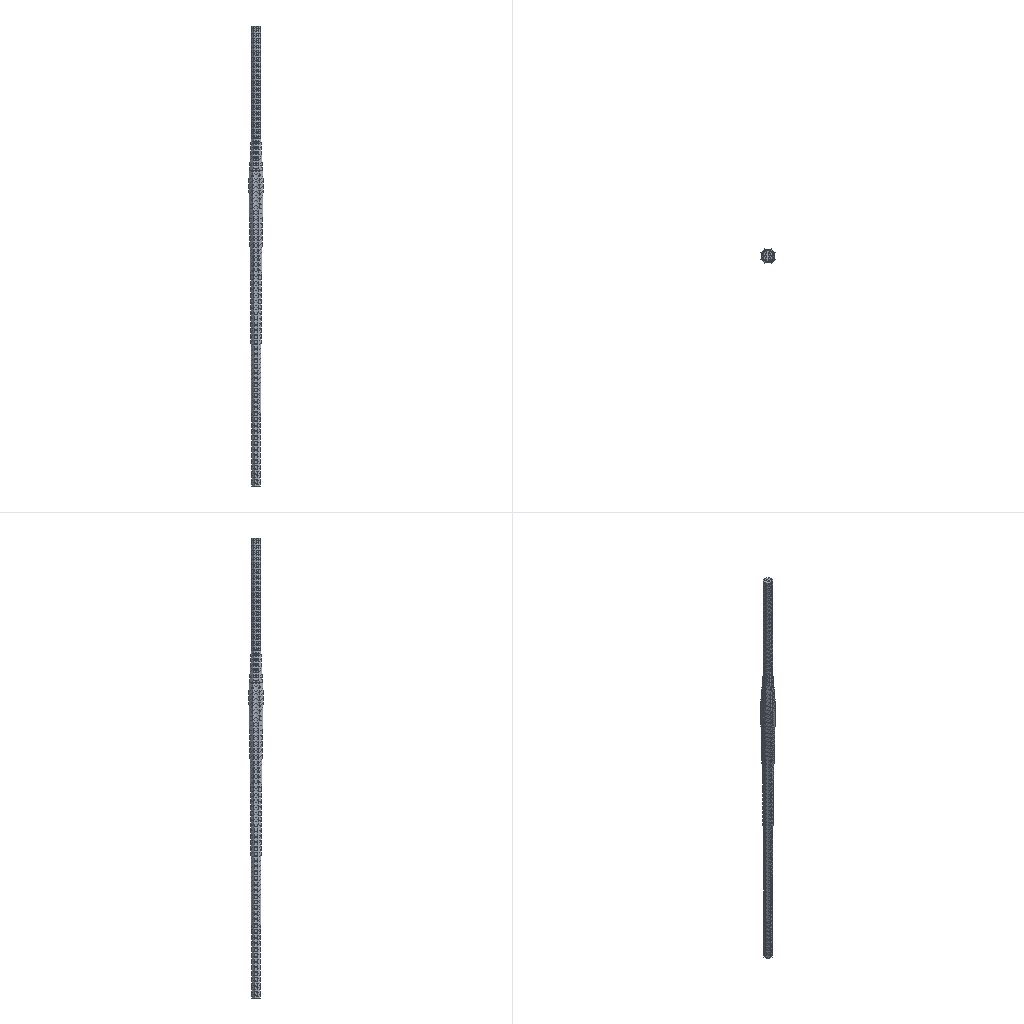Simulation study | abaqus
Set-up summary:
category,name,step,type,value,unit,region
solver,abaqus
solver,version,,,Abaqus/Explicit 2020
units,not stated in the deck,,not stated
analysis,deck,,transient,transient
load_step,Step-1,Step-1,transient,nlgeom=True
contact,interactions,,,general=0 pairs=1 ties=0
load_step,requested,,,1
mesh,nodes,,,15796
mesh,elements,,,8700
element_type,R3D3,,rigid,14
element_type,R3D4,,rigid,1363
element_type,C3D10M,,solid,7323
load,load commands in deck,,count,1
bc,support commands in deck,,count,6
material,MATERIAL-1,,in results
check,setup vs results,,match,"per instance, exact: element labels, types and connectivity; labels of the nodes the elements use; coordinates of those nodes at SINGLE_PRECISION in 1 of 2 instance(s)"
Abaqus input file, long lists of numbers shortened:
*Heading
** Job name: Job-3 Model name: Model-1-Copy2
** Generated by: Abaqus/CAE 2020
*Preprint, echo=NO, model=NO, history=NO, contact=NO
**
** PARTS
**
*Part, name="Men Surface v1"
*Node
      1,         -60.,  -26.267,   112.347
      2,          60.,  -26.267,   112.347
** (1370 more lines like these left out)
*Element, type=R3D4
 1,   1,  13, 183,  30
 2,  13,  14, 184, 183
** (1361 more lines like these left out)
*Element, type=R3D3
604,  837,  861,  875
605, 1000,  919,  815
** (12 more lines like these left out)
*Node
   1373,           0.,  -142.754,  -4.552
*Nset, nset="Men Surface v1-RefPt_", internal
1373,
*Elset, elset="Men Surface v1", generate
    1,  1377,     1
*End Part
**
*Part, name="Shinai Koto v4"
*Node
      1,         -13.,           0.,           0.
      2,   5.495,  -11.781,         300.
** (14421 more lines like these left out)
*Element, type=C3D10M
   1,  2089,  1420,  2090,  1417,  2506,  2505,  2504,  2508,  2507,  2509
   2,  2089,  2090,  2091,  2092,  2504,  2511,  2510,  2513,  2512,  2514
** (7321 more lines like these left out)
*Nset, nset=Set-4, generate
     1,  14423,      1
*Elset, elset=Set-4, generate
    1,  7323,     1
*Orientation, name=Ori-1
1., 0., 0., 0., 1., 0.
1, 0.
** Section: Section-1
*Solid Section, elset=Set-4, orientation=Ori-1, material=Material-1
,
*End Part
**
**
** ASSEMBLY
**
*Assembly, name=Assembly
**
*Instance, name="Men Surface v1-1", part="Men Surface v1"
1.74822750328583e-14, -167.849, 62.883
1.74822750328583e-14, -167.849, 62.883, 1.75414209299603e-14, -166.883, 63.142,         180.
*End Instance
**
*Instance, name="Shinai Koto v4-1", part="Shinai Koto v4"
          0.,           0.,         950.
          0.,           0.,         950.,           1.,           0.,         950.,         180.
*End Instance
**
*Nset, nset=Set-4, instance="Men Surface v1-1"
 1373,
*Nset, nset=Set-5, instance="Shinai Koto v4-1"
     4,     5,     8,     9,    12,    13,    20,    21,    26,    27,    28,    29,    30,    31,    32,    33
    34,    35,    36,    37,    38,    39,    40,    41,    42,    43,    44,    45,    46,    47,    48,    49
** (397 more lines like these left out)
*Elset, elset=Set-5, instance="Shinai Koto v4-1"
   74,  145,  149,  150,  152,  154,  155,  156,  170,  172,  175,  176,  178,  183,  184,  186
  187,  188,  190,  191,  192,  195,  197,  206,  207,  210,  211,  212,  213,  215,  216,  217
** (194 more lines like these left out)
*Nset, nset=Set-6, instance="Shinai Koto v4-1"
     1,     2,     3,     6,     7,    10,    11,    18,    19,    22,    23,    24,    25,   106,   107,   108
   109,   110,   111,   112,   113,   114,   115,   116,   181,   182,   183,   184,   185,   186,   187,   188
** (71 more lines like these left out)
*Elset, elset=Set-6, instance="Shinai Koto v4-1"
   58,   80,   92,  102,  121,  331,  422,  555,  606,  614,  701,  723,  813, 1010, 1070, 1108
 1201, 1368, 1370, 1381, 1385, 1535, 1542, 1651, 1807, 1834, 2154, 2190, 2191, 2199, 2291, 2295
** (34 more lines like these left out)
*Nset, nset=Set-7, instance="Shinai Koto v4-1"
     1,   106,   107,   108,   109,   110,   111,   112,   113,   114,   115,   116,  1771,  1772,  1773,  1774
  1775,  1776,  1777,  8271,  8284,  8288,  8291,  8772,  8775,  8783,  8810,  8816,  9594,  9596,  9598,  9639
** (2 more lines like these left out)
*Elset, elset=Set-7, instance="Shinai Koto v4-1"
 2154, 2461, 2526, 2534, 2898, 2961, 2986, 2988, 2992, 2996, 2997, 3004, 3005, 3010, 3012, 3016
 3025, 3027, 3034, 3042, 3051, 3633, 3635, 3669
*Elset, elset=_m_Surf-1_SPOS, internal, instance="Men Surface v1-1", generate
    1,  1377,     1
*Surface, type=ELEMENT, name=m_Surf-1
_m_Surf-1_SPOS, SPOS
*Elset, elset=_s_Surf-3_S3, internal, instance="Shinai Koto v4-1"
   47,   58,   74,  102,  121,  145,  149,  150,  152,  154,  155,  156,  160,  161,  165,  168
  170,  172,  175,  176,  178,  183,  184,  186,  187,  188,  190,  191,  192,  195,  206,  207
** (245 more lines like these left out)
*Elset, elset=_s_Surf-3_S2, internal, instance="Shinai Koto v4-1"
  289,  751,  759,  885,  935, 1538, 1974, 2199, 2295, 2330, 2377, 2487, 2507, 2731, 2734, 2891
 3137, 3167, 3267, 3284, 3349, 3364, 3373, 3388, 3450, 3542, 3700, 3747, 3778, 3850, 3943, 3957
** (3 more lines like these left out)
*Elset, elset=_s_Surf-3_S1, internal, instance="Shinai Koto v4-1"
  285,  286,  297,  817, 1201, 1428, 2132, 2155, 2276, 2371, 2563, 2592, 2599, 2726, 2933, 3082
 3132, 3149, 3192, 3257, 3262, 3287, 3358, 3373, 3399, 3420, 3453, 3454, 3455, 3457, 3594, 3599
** (4 more lines like these left out)
*Elset, elset=_s_Surf-3_S4, internal, instance="Shinai Koto v4-1"
   80,   92,  197,  295,  556,  562,  589,  606,  614,  701,  715, 1010, 1070, 1535, 1613, 1651
 1807, 1834, 2133, 2207, 2291, 2346, 2358, 2360, 2367, 2373, 2401, 2420, 2502, 2511, 2624, 2821
** (4 more lines like these left out)
*Surface, type=ELEMENT, name=s_Surf-3
_s_Surf-3_S3, S3
_s_Surf-3_S2, S2
_s_Surf-3_S4, S4
_s_Surf-3_S1, S1
*Rigid Body, ref node="Men Surface v1-1"."Men Surface v1-RefPt_", elset="Men Surface v1-1"."Men Surface v1"
*End Assembly
**
** MATERIALS
**
*Material, name=Material-1
*Density
 1e-09,
*Elastic, type=ENGINEERING CONSTANTS
20000., 2485.,20000.,  0.35,  0.35,   0.3, 7588., 1000.
 1000.,
**
** INTERACTION PROPERTIES
**
*Surface Interaction, name=IntProp-1
*Friction
 0.1,
*Surface Behavior, pressure-overclosure=HARD
**
** PREDEFINED FIELDS
**
** Name: Predefined Field-1   Type: Velocity
*Initial Conditions, type=ROTATING VELOCITY
Set-5, -100.,  ,  ,  ,
0., 0., 950., 1., 0., 950.,
** ----------------------------------------------------------------
**
** STEP: Step-1
**
*Step, name=Step-1, nlgeom=YES
*Dynamic, Explicit
, 0.002
*Bulk Viscosity
0.06, 1.2
**
** BOUNDARY CONDITIONS
**
** Name: BC-1 Type: 位移/转角
*Boundary
Set-7, 1, 1
Set-7, 2, 2
Set-7, 3, 3
Set-7, 5, 5
Set-7, 6, 6
** Name: BC-2 Type: 对称/反对称/完全固定
*Boundary
Set-4, ENCASTRE
**
** INTERACTIONS
**
** Interaction: Int-1
*Contact Pair, interaction=IntProp-1, mechanical constraint=KINEMATIC, cpset=Int-1
m_Surf-1, s_Surf-3
**
** OUTPUT REQUESTS
**
*Restart, write, number interval=1, time marks=NO
**
** FIELD OUTPUT: F-Output-1
**
*Output, field, number interval=100
*Node Output
A, CF, RF, RM, RT, U, V
*Element Output, directions=YES
E, EVF, LE, MISES, MISESMAX, PE, PEEQ, PEEQVAVG, PEVAVG, S, SF, SSAVG, SVAVG
*Contact Output
CDISP, CSTRESS
**
** HISTORY OUTPUT: H-Output-1
**
*Output, history, variable=PRESELECT
*End Step
Results summary:
result,step,Step-1,completed,increments=233612 time=0.002/0.002
result,analysis,,,transient
result,last_loadstep,,,1
result,analysis steps,,count,1
result,primary field,,,U
result,reaction total,,FX,9.482,model units
result,reaction total,,FY,2254.276,model units
result,reaction total,,FZ,329.023,model units